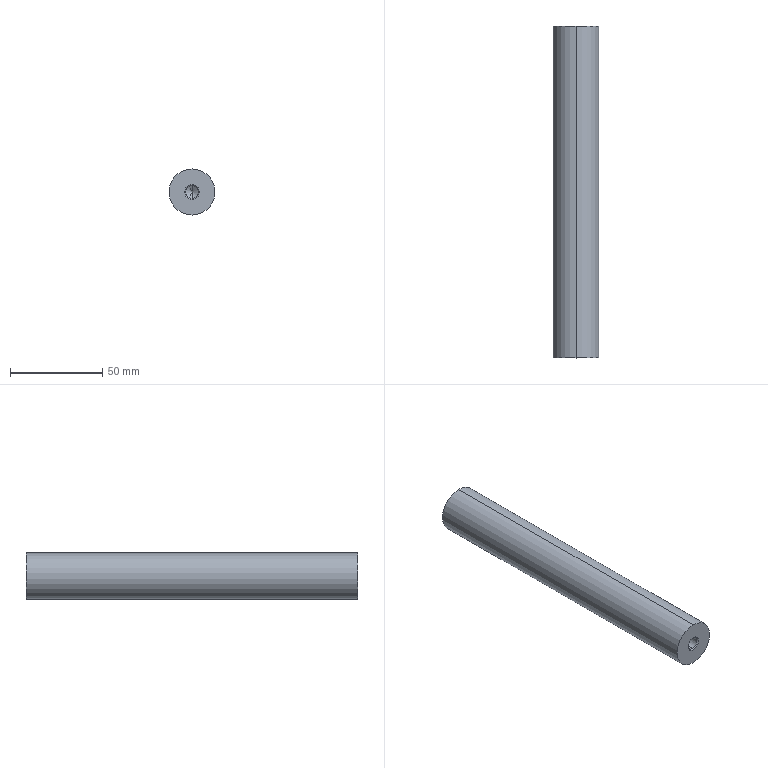Part | STEP file | A14-006 | 1 solid | 16 faces | box 25 x 180 x 25 mm | volume 86683 mm3 | cone 8 | cylinder 6 | plane 2 | commonest cylinder face diameters 6.8 x4 25 x2
STEP:
#1=CARTESIAN_POINT('',(0.,0.,0.));
#2=DIRECTION('',(0.,0.,1.));
#3=DIRECTION('',(1.,0.,0.));
#4=AXIS2_PLACEMENT_3D('',#1,#2,#3);
#5=CARTESIAN_POINT('',(0.,89.375,3.4));
#6=VERTEX_POINT('',#5);
#7=CARTESIAN_POINT('',(0.,90.,4.025));
#8=VERTEX_POINT('',#7);
#9=CARTESIAN_POINT('',(0.,90.,4.025));
#10=DIRECTION('',(0.,0.7071,0.7071));
#11=VECTOR('',#10,1.);
#12=LINE('',#9,#11);
#13=CARTESIAN_POINT('',(0.,90.,0.));
#14=DIRECTION('',(0.,1.,0.));
#15=DIRECTION('',(0.,0.,1.));
#16=AXIS2_PLACEMENT_3D('',#13,#14,#15);
#17=CONICAL_SURFACE('',#16,4.025,0.7854);
#18=CARTESIAN_POINT('',(6.283,0.));
#19=DIRECTION('',(0.,1.));
#20=VECTOR('',#19,1.);
#21=LINE('',#18,#20);
#22=(GEOMETRIC_REPRESENTATION_CONTEXT(2)PARAMETRIC_REPRESENTATION_CONTEXT()REPRESENTATION_CONTEXT('',''));
#23=DEFINITIONAL_REPRESENTATION('',(#21),#22);
#24=PCURVE('',#17,#23);
#25=CARTESIAN_POINT('',(0.,90.,0.));
#26=DIRECTION('',(0.,1.,0.));
#27=DIRECTION('',(0.,0.,1.));
#28=AXIS2_PLACEMENT_3D('',#25,#26,#27);
#29=CONICAL_SURFACE('',#28,4.025,0.7854);
#30=CARTESIAN_POINT('',(0.,0.));
#31=DIRECTION('',(0.,1.));
#32=VECTOR('',#31,1.);
#33=LINE('',#30,#32);
#34=(GEOMETRIC_REPRESENTATION_CONTEXT(2)PARAMETRIC_REPRESENTATION_CONTEXT()REPRESENTATION_CONTEXT('',''));
#35=DEFINITIONAL_REPRESENTATION('',(#33),#34);
#36=PCURVE('',#29,#35);
#37=SURFACE_CURVE('',#12,(#24,#36),.PCURVE_S1.);
#38=EDGE_CURVE('',#6,#8,#37,.T.);
#39=ORIENTED_EDGE('',*,*,#38,.T.);
#40=CARTESIAN_POINT('',(0.,90.,-4.025));
#41=VERTEX_POINT('',#40);
#42=CARTESIAN_POINT('',(0.,90.,0.));
#43=DIRECTION('',(0.,1.,0.));
#44=DIRECTION('',(0.,0.,1.));
#45=AXIS2_PLACEMENT_3D('',#42,#43,#44);
#46=CIRCLE('',#45,4.025);
#47=CARTESIAN_POINT('',(0.,0.));
#48=DIRECTION('',(1.,0.));
#49=VECTOR('',#48,1.);
#50=LINE('',#47,#49);
#51=(GEOMETRIC_REPRESENTATION_CONTEXT(2)PARAMETRIC_REPRESENTATION_CONTEXT()REPRESENTATION_CONTEXT('',''));
#52=DEFINITIONAL_REPRESENTATION('',(#50),#51);
#53=PCURVE('',#17,#52);
#54=CARTESIAN_POINT('',(0.,90.,0.));
#55=DIRECTION('',(0.,1.,0.));
#56=DIRECTION('',(0.,0.,1.));
#57=AXIS2_PLACEMENT_3D('',#54,#55,#56);
#58=PLANE('',#57);
#59=CARTESIAN_POINT('',(0.,0.));
#60=DIRECTION('',(1.,0.));
#61=AXIS2_PLACEMENT_2D('',#59,#60);
#62=CIRCLE('',#61,4.025);
#63=(GEOMETRIC_REPRESENTATION_CONTEXT(2)PARAMETRIC_REPRESENTATION_CONTEXT()REPRESENTATION_CONTEXT('',''));
#64=DEFINITIONAL_REPRESENTATION('',(#62),#63);
#65=PCURVE('',#58,#64);
#66=SURFACE_CURVE('',#46,(#53,#65),.PCURVE_S1.);
#67=EDGE_CURVE('',#41,#8,#66,.T.);
#68=ORIENTED_EDGE('',*,*,#67,.F.);
#69=CARTESIAN_POINT('',(0.,89.375,-3.4));
#70=VERTEX_POINT('',#69);
#71=CARTESIAN_POINT('',(0.,90.,-4.025));
#72=DIRECTION('',(0.,0.7071,-0.7071));
#73=VECTOR('',#72,1.);
#74=LINE('',#71,#73);
#75=CARTESIAN_POINT('',(3.142,0.));
#76=DIRECTION('',(0.,1.));
#77=VECTOR('',#76,1.);
#78=LINE('',#75,#77);
#79=(GEOMETRIC_REPRESENTATION_CONTEXT(2)PARAMETRIC_REPRESENTATION_CONTEXT()REPRESENTATION_CONTEXT('',''));
#80=DEFINITIONAL_REPRESENTATION('',(#78),#79);
#81=PCURVE('',#17,#80);
#82=CARTESIAN_POINT('',(3.142,0.));
#83=DIRECTION('',(0.,1.));
#84=VECTOR('',#83,1.);
#85=LINE('',#82,#84);
#86=(GEOMETRIC_REPRESENTATION_CONTEXT(2)PARAMETRIC_REPRESENTATION_CONTEXT()REPRESENTATION_CONTEXT('',''));
#87=DEFINITIONAL_REPRESENTATION('',(#85),#86);
#88=PCURVE('',#29,#87);
#89=SURFACE_CURVE('',#74,(#81,#88),.PCURVE_S1.);
#90=EDGE_CURVE('',#70,#41,#89,.T.);
#91=ORIENTED_EDGE('',*,*,#90,.F.);
#92=CARTESIAN_POINT('',(0.,89.375,0.));
#93=DIRECTION('',(0.,1.,0.));
#94=DIRECTION('',(0.,0.,1.));
#95=AXIS2_PLACEMENT_3D('',#92,#93,#94);
#96=CIRCLE('',#95,3.4);
#97=CARTESIAN_POINT('',(0.,-0.625));
#98=DIRECTION('',(1.,0.));
#99=VECTOR('',#98,1.);
#100=LINE('',#97,#99);
#101=(GEOMETRIC_REPRESENTATION_CONTEXT(2)PARAMETRIC_REPRESENTATION_CONTEXT()REPRESENTATION_CONTEXT('',''));
#102=DEFINITIONAL_REPRESENTATION('',(#100),#101);
#103=PCURVE('',#17,#102);
#104=CARTESIAN_POINT('',(0.,90.,0.));
#105=DIRECTION('',(0.,1.,0.));
#106=DIRECTION('',(0.,0.,1.));
#107=AXIS2_PLACEMENT_3D('',#104,#105,#106);
#108=CYLINDRICAL_SURFACE('',#107,3.4);
#109=CARTESIAN_POINT('',(0.,-0.625));
#110=DIRECTION('',(1.,0.));
#111=VECTOR('',#110,1.);
#112=LINE('',#109,#111);
#113=(GEOMETRIC_REPRESENTATION_CONTEXT(2)PARAMETRIC_REPRESENTATION_CONTEXT()REPRESENTATION_CONTEXT('',''));
#114=DEFINITIONAL_REPRESENTATION('',(#112),#113);
#115=PCURVE('',#108,#114);
#116=SURFACE_CURVE('',#96,(#103,#115),.PCURVE_S1.);
#117=EDGE_CURVE('',#70,#6,#116,.T.);
#118=ORIENTED_EDGE('',*,*,#117,.T.);
#119=EDGE_LOOP('',(#39,#68,#91,#118));
#120=FACE_BOUND('',#119,.F.);
#121=ADVANCED_FACE('',(#120),#17,.F.);
#122=CARTESIAN_POINT('',(0.,67.75,3.4));
#123=VERTEX_POINT('',#122);
#124=CARTESIAN_POINT('',(0.,90.,3.4));
#125=DIRECTION('',(0.,1.,0.));
#126=VECTOR('',#125,1.);
#127=LINE('',#124,#126);
#128=CARTESIAN_POINT('',(6.283,0.));
#129=DIRECTION('',(0.,1.));
#130=VECTOR('',#129,1.);
#131=LINE('',#128,#130);
#132=(GEOMETRIC_REPRESENTATION_CONTEXT(2)PARAMETRIC_REPRESENTATION_CONTEXT()REPRESENTATION_CONTEXT('',''));
#133=DEFINITIONAL_REPRESENTATION('',(#131),#132);
#134=PCURVE('',#108,#133);
#135=CARTESIAN_POINT('',(0.,90.,0.));
#136=DIRECTION('',(0.,1.,0.));
#137=DIRECTION('',(0.,0.,1.));
#138=AXIS2_PLACEMENT_3D('',#135,#136,#137);
#139=CYLINDRICAL_SURFACE('',#138,3.4);
#140=CARTESIAN_POINT('',(0.,0.));
#141=DIRECTION('',(0.,1.));
#142=VECTOR('',#141,1.);
#143=LINE('',#140,#142);
#144=(GEOMETRIC_REPRESENTATION_CONTEXT(2)PARAMETRIC_REPRESENTATION_CONTEXT()REPRESENTATION_CONTEXT('',''));
#145=DEFINITIONAL_REPRESENTATION('',(#143),#144);
#146=PCURVE('',#139,#145);
#147=SURFACE_CURVE('',#127,(#134,#146),.PCURVE_S1.);
#148=EDGE_CURVE('',#123,#6,#147,.T.);
#149=ORIENTED_EDGE('',*,*,#148,.T.);
#150=ORIENTED_EDGE('',*,*,#117,.F.);
#151=CARTESIAN_POINT('',(0.,67.75,-3.4));
#152=VERTEX_POINT('',#151);
#153=CARTESIAN_POINT('',(0.,90.,-3.4));
#154=DIRECTION('',(0.,1.,0.));
#155=VECTOR('',#154,1.);
#156=LINE('',#153,#155);
#157=CARTESIAN_POINT('',(3.142,0.));
#158=DIRECTION('',(0.,1.));
#159=VECTOR('',#158,1.);
#160=LINE('',#157,#159);
#161=(GEOMETRIC_REPRESENTATION_CONTEXT(2)PARAMETRIC_REPRESENTATION_CONTEXT()REPRESENTATION_CONTEXT('',''));
#162=DEFINITIONAL_REPRESENTATION('',(#160),#161);
#163=PCURVE('',#108,#162);
#164=CARTESIAN_POINT('',(3.142,0.));
#165=DIRECTION('',(0.,1.));
#166=VECTOR('',#165,1.);
#167=LINE('',#164,#166);
#168=(GEOMETRIC_REPRESENTATION_CONTEXT(2)PARAMETRIC_REPRESENTATION_CONTEXT()REPRESENTATION_CONTEXT('',''));
#169=DEFINITIONAL_REPRESENTATION('',(#167),#168);
#170=PCURVE('',#139,#169);
#171=SURFACE_CURVE('',#156,(#163,#170),.PCURVE_S1.);
#172=EDGE_CURVE('',#152,#70,#171,.T.);
#173=ORIENTED_EDGE('',*,*,#172,.F.);
#174=CARTESIAN_POINT('',(0.,67.75,0.));
#175=DIRECTION('',(0.,1.,0.));
#176=DIRECTION('',(0.,0.,1.));
#177=AXIS2_PLACEMENT_3D('',#174,#175,#176);
#178=CIRCLE('',#177,3.4);
#179=CARTESIAN_POINT('',(0.,-22.25));
#180=DIRECTION('',(1.,0.));
#181=VECTOR('',#180,1.);
#182=LINE('',#179,#181);
#183=(GEOMETRIC_REPRESENTATION_CONTEXT(2)PARAMETRIC_REPRESENTATION_CONTEXT()REPRESENTATION_CONTEXT('',''));
#184=DEFINITIONAL_REPRESENTATION('',(#182),#183);
#185=PCURVE('',#108,#184);
#186=CARTESIAN_POINT('',(0.,67.75,0.));
#187=DIRECTION('',(0.,1.,0.));
#188=DIRECTION('',(0.,0.,1.));
#189=AXIS2_PLACEMENT_3D('',#186,#187,#188);
#190=CONICAL_SURFACE('',#189,3.4,1.03);
#191=CARTESIAN_POINT('',(0.,0.));
#192=DIRECTION('',(1.,0.));
#193=VECTOR('',#192,1.);
#194=LINE('',#191,#193);
#195=(GEOMETRIC_REPRESENTATION_CONTEXT(2)PARAMETRIC_REPRESENTATION_CONTEXT()REPRESENTATION_CONTEXT('',''));
#196=DEFINITIONAL_REPRESENTATION('',(#194),#195);
#197=PCURVE('',#190,#196);
#198=SURFACE_CURVE('',#178,(#185,#197),.PCURVE_S1.);
#199=EDGE_CURVE('',#152,#123,#198,.T.);
#200=ORIENTED_EDGE('',*,*,#199,.T.);
#201=EDGE_LOOP('',(#149,#150,#173,#200));
#202=FACE_BOUND('',#201,.F.);
#203=ADVANCED_FACE('',(#202),#108,.F.);
#204=ORIENTED_EDGE('',*,*,#199,.F.);
#205=CARTESIAN_POINT('',(0.,65.707,0.));
#206=VERTEX_POINT('',#205);
#207=CARTESIAN_POINT('',(0.,67.75,-3.4));
#208=DIRECTION('',(0.,0.515,-0.8572));
#209=VECTOR('',#208,1.);
#210=LINE('',#207,#209);
#211=CARTESIAN_POINT('',(3.142,-2.043));
#212=CARTESIAN_POINT('',(3.142,-2.012));
#213=CARTESIAN_POINT('',(3.142,-1.95));
#214=CARTESIAN_POINT('',(3.142,-1.857));
#215=CARTESIAN_POINT('',(3.142,-1.764));
#216=CARTESIAN_POINT('',(3.142,-1.671));
#217=CARTESIAN_POINT('',(3.142,-1.579));
#218=CARTESIAN_POINT('',(3.142,-1.486));
#219=CARTESIAN_POINT('',(3.142,-1.393));
#220=CARTESIAN_POINT('',(3.142,-1.3));
#221=CARTESIAN_POINT('',(3.142,-1.207));
#222=CARTESIAN_POINT('',(3.142,-1.114));
#223=CARTESIAN_POINT('',(3.142,-1.021));
#224=CARTESIAN_POINT('',(3.142,-0.9286));
#225=CARTESIAN_POINT('',(3.142,-0.8357));
#226=CARTESIAN_POINT('',(3.142,-0.7429));
#227=CARTESIAN_POINT('',(3.142,-0.65));
#228=CARTESIAN_POINT('',(3.142,-0.5572));
#229=CARTESIAN_POINT('',(3.142,-0.4643));
#230=CARTESIAN_POINT('',(3.142,-0.3714));
#231=CARTESIAN_POINT('',(3.142,-0.2786));
#232=CARTESIAN_POINT('',(3.142,-0.1857));
#233=CARTESIAN_POINT('',(3.142,-0.09286));
#234=CARTESIAN_POINT('',(3.142,-0.03095));
#235=CARTESIAN_POINT('',(3.142,0.));
#236=B_SPLINE_CURVE_WITH_KNOTS('',3,(#211,#212,#213,#214,#215,#216,#217,#218,#219,#220,#221,#222,#223,#224,#225,#226,#227,#228,#229,#230,#231,#232,#233,#234,#235),.UNSPECIFIED.,.F.,.F.,(4,1,1,1,1,1,1,1,1,1,1,1,1,1,1,1,1,1,1,1,1,1,4),(-3.967,-3.786,-3.606,-3.426,-3.245,-3.065,-2.885,-2.704,-2.524,-2.344,-2.164,-1.983,-1.803,-1.623,-1.442,-1.262,-1.082,-0.9015,-0.7212,-0.5409,-0.3606,-0.1803,0.),.UNSPECIFIED.);
#237=(GEOMETRIC_REPRESENTATION_CONTEXT(2)PARAMETRIC_REPRESENTATION_CONTEXT()REPRESENTATION_CONTEXT('',''));
#238=DEFINITIONAL_REPRESENTATION('',(#236),#237);
#239=PCURVE('',#190,#238);
#240=CARTESIAN_POINT('',(0.,67.75,0.));
#241=DIRECTION('',(0.,1.,0.));
#242=DIRECTION('',(0.,0.,1.));
#243=AXIS2_PLACEMENT_3D('',#240,#241,#242);
#244=CONICAL_SURFACE('',#243,3.4,1.03);
#245=CARTESIAN_POINT('',(3.142,-2.043));
#246=CARTESIAN_POINT('',(3.142,-2.012));
#247=CARTESIAN_POINT('',(3.142,-1.95));
#248=CARTESIAN_POINT('',(3.142,-1.857));
#249=CARTESIAN_POINT('',(3.142,-1.764));
#250=CARTESIAN_POINT('',(3.142,-1.671));
#251=CARTESIAN_POINT('',(3.142,-1.579));
#252=CARTESIAN_POINT('',(3.142,-1.486));
#253=CARTESIAN_POINT('',(3.142,-1.393));
#254=CARTESIAN_POINT('',(3.142,-1.3));
#255=CARTESIAN_POINT('',(3.142,-1.207));
#256=CARTESIAN_POINT('',(3.142,-1.114));
#257=CARTESIAN_POINT('',(3.142,-1.021));
#258=CARTESIAN_POINT('',(3.142,-0.9286));
#259=CARTESIAN_POINT('',(3.142,-0.8357));
#260=CARTESIAN_POINT('',(3.142,-0.7429));
#261=CARTESIAN_POINT('',(3.142,-0.65));
#262=CARTESIAN_POINT('',(3.142,-0.5572));
#263=CARTESIAN_POINT('',(3.142,-0.4643));
#264=CARTESIAN_POINT('',(3.142,-0.3714));
#265=CARTESIAN_POINT('',(3.142,-0.2786));
#266=CARTESIAN_POINT('',(3.142,-0.1857));
#267=CARTESIAN_POINT('',(3.142,-0.09286));
#268=CARTESIAN_POINT('',(3.142,-0.03095));
#269=CARTESIAN_POINT('',(3.142,0.));
#270=B_SPLINE_CURVE_WITH_KNOTS('',3,(#245,#246,#247,#248,#249,#250,#251,#252,#253,#254,#255,#256,#257,#258,#259,#260,#261,#262,#263,#264,#265,#266,#267,#268,#269),.UNSPECIFIED.,.F.,.F.,(4,1,1,1,1,1,1,1,1,1,1,1,1,1,1,1,1,1,1,1,1,1,4),(-3.967,-3.786,-3.606,-3.426,-3.245,-3.065,-2.885,-2.704,-2.524,-2.344,-2.164,-1.983,-1.803,-1.623,-1.442,-1.262,-1.082,-0.9015,-0.7212,-0.5409,-0.3606,-0.1803,0.),.UNSPECIFIED.);
#271=(GEOMETRIC_REPRESENTATION_CONTEXT(2)PARAMETRIC_REPRESENTATION_CONTEXT()REPRESENTATION_CONTEXT('',''));
#272=DEFINITIONAL_REPRESENTATION('',(#270),#271);
#273=PCURVE('',#244,#272);
#274=SURFACE_CURVE('',#210,(#239,#273),.PCURVE_S1.);
#275=EDGE_CURVE('',#206,#152,#274,.T.);
#276=ORIENTED_EDGE('',*,*,#275,.F.);
#277=CARTESIAN_POINT('',(0.,67.75,3.4));
#278=DIRECTION('',(0.,0.515,0.8572));
#279=VECTOR('',#278,1.);
#280=LINE('',#277,#279);
#281=CARTESIAN_POINT('',(6.283,-2.043));
#282=CARTESIAN_POINT('',(6.283,-2.012));
#283=CARTESIAN_POINT('',(6.283,-1.95));
#284=CARTESIAN_POINT('',(6.283,-1.857));
#285=CARTESIAN_POINT('',(6.283,-1.764));
#286=CARTESIAN_POINT('',(6.283,-1.671));
#287=CARTESIAN_POINT('',(6.283,-1.579));
#288=CARTESIAN_POINT('',(6.283,-1.486));
#289=CARTESIAN_POINT('',(6.283,-1.393));
#290=CARTESIAN_POINT('',(6.283,-1.3));
#291=CARTESIAN_POINT('',(6.283,-1.207));
#292=CARTESIAN_POINT('',(6.283,-1.114));
#293=CARTESIAN_POINT('',(6.283,-1.021));
#294=CARTESIAN_POINT('',(6.283,-0.9286));
#295=CARTESIAN_POINT('',(6.283,-0.8357));
#296=CARTESIAN_POINT('',(6.283,-0.7429));
#297=CARTESIAN_POINT('',(6.283,-0.65));
#298=CARTESIAN_POINT('',(6.283,-0.5572));
#299=CARTESIAN_POINT('',(6.283,-0.4643));
#300=CARTESIAN_POINT('',(6.283,-0.3714));
#301=CARTESIAN_POINT('',(6.283,-0.2786));
#302=CARTESIAN_POINT('',(6.283,-0.1857));
#303=CARTESIAN_POINT('',(6.283,-0.09286));
#304=CARTESIAN_POINT('',(6.283,-0.03095));
#305=CARTESIAN_POINT('',(6.283,0.));
#306=B_SPLINE_CURVE_WITH_KNOTS('',3,(#281,#282,#283,#284,#285,#286,#287,#288,#289,#290,#291,#292,#293,#294,#295,#296,#297,#298,#299,#300,#301,#302,#303,#304,#305),.UNSPECIFIED.,.F.,.F.,(4,1,1,1,1,1,1,1,1,1,1,1,1,1,1,1,1,1,1,1,1,1,4),(-3.967,-3.786,-3.606,-3.426,-3.245,-3.065,-2.885,-2.704,-2.524,-2.344,-2.164,-1.983,-1.803,-1.623,-1.442,-1.262,-1.082,-0.9015,-0.7212,-0.5409,-0.3606,-0.1803,0.),.UNSPECIFIED.);
#307=(GEOMETRIC_REPRESENTATION_CONTEXT(2)PARAMETRIC_REPRESENTATION_CONTEXT()REPRESENTATION_CONTEXT('',''));
#308=DEFINITIONAL_REPRESENTATION('',(#306),#307);
#309=PCURVE('',#190,#308);
#310=CARTESIAN_POINT('',(0.,-2.043));
#311=CARTESIAN_POINT('',(0.,-2.012));
#312=CARTESIAN_POINT('',(0.,-1.95));
#313=CARTESIAN_POINT('',(0.,-1.857));
#314=CARTESIAN_POINT('',(0.,-1.764));
#315=CARTESIAN_POINT('',(0.,-1.671));
#316=CARTESIAN_POINT('',(0.,-1.579));
#317=CARTESIAN_POINT('',(0.,-1.486));
#318=CARTESIAN_POINT('',(0.,-1.393));
#319=CARTESIAN_POINT('',(0.,-1.3));
#320=CARTESIAN_POINT('',(0.,-1.207));
#321=CARTESIAN_POINT('',(0.,-1.114));
#322=CARTESIAN_POINT('',(0.,-1.021));
#323=CARTESIAN_POINT('',(0.,-0.9286));
#324=CARTESIAN_POINT('',(0.,-0.8357));
#325=CARTESIAN_POINT('',(0.,-0.7429));
#326=CARTESIAN_POINT('',(0.,-0.65));
#327=CARTESIAN_POINT('',(0.,-0.5572));
#328=CARTESIAN_POINT('',(0.,-0.4643));
#329=CARTESIAN_POINT('',(0.,-0.3714));
#330=CARTESIAN_POINT('',(0.,-0.2786));
#331=CARTESIAN_POINT('',(0.,-0.1857));
#332=CARTESIAN_POINT('',(0.,-0.09286));
#333=CARTESIAN_POINT('',(0.,-0.03095));
#334=CARTESIAN_POINT('',(0.,0.));
#335=B_SPLINE_CURVE_WITH_KNOTS('',3,(#310,#311,#312,#313,#314,#315,#316,#317,#318,#319,#320,#321,#322,#323,#324,#325,#326,#327,#328,#329,#330,#331,#332,#333,#334),.UNSPECIFIED.,.F.,.F.,(4,1,1,1,1,1,1,1,1,1,1,1,1,1,1,1,1,1,1,1,1,1,4),(-3.967,-3.786,-3.606,-3.426,-3.245,-3.065,-2.885,-2.704,-2.524,-2.344,-2.164,-1.983,-1.803,-1.623,-1.442,-1.262,-1.082,-0.9015,-0.7212,-0.5409,-0.3606,-0.1803,0.),.UNSPECIFIED.);
#336=(GEOMETRIC_REPRESENTATION_CONTEXT(2)PARAMETRIC_REPRESENTATION_CONTEXT()REPRESENTATION_CONTEXT('',''));
#337=DEFINITIONAL_REPRESENTATION('',(#335),#336);
#338=PCURVE('',#244,#337);
#339=SURFACE_CURVE('',#280,(#309,#338),.PCURVE_S1.);
#340=EDGE_CURVE('',#206,#123,#339,.T.);
#341=ORIENTED_EDGE('',*,*,#340,.T.);
#342=EDGE_LOOP('',(#204,#276,#341));
#343=FACE_BOUND('',#342,.F.);
#344=ADVANCED_FACE('',(#343),#190,.F.);
#345=CARTESIAN_POINT('',(0.,-89.375,-3.4));
#346=VERTEX_POINT('',#345);
#347=CARTESIAN_POINT('',(0.,-90.,-4.025));
#348=VERTEX_POINT('',#347);
#349=CARTESIAN_POINT('',(0.,-90.,-4.025));
#350=DIRECTION('',(0.,-0.7071,-0.7071));
#351=VECTOR('',#350,1.);
#352=LINE('',#349,#351);
#353=CARTESIAN_POINT('',(0.,-90.,0.));
#354=DIRECTION('',(0.,-1.,0.));
#355=DIRECTION('',(0.,0.,-1.));
#356=AXIS2_PLACEMENT_3D('',#353,#354,#355);
#357=CONICAL_SURFACE('',#356,4.025,0.7854);
#358=CARTESIAN_POINT('',(6.283,0.));
#359=DIRECTION('',(0.,1.));
#360=VECTOR('',#359,1.);
#361=LINE('',#358,#360);
#362=(GEOMETRIC_REPRESENTATION_CONTEXT(2)PARAMETRIC_REPRESENTATION_CONTEXT()REPRESENTATION_CONTEXT('',''));
#363=DEFINITIONAL_REPRESENTATION('',(#361),#362);
#364=PCURVE('',#357,#363);
#365=CARTESIAN_POINT('',(0.,-90.,0.));
#366=DIRECTION('',(0.,-1.,0.));
#367=DIRECTION('',(0.,0.,-1.));
#368=AXIS2_PLACEMENT_3D('',#365,#366,#367);
#369=CONICAL_SURFACE('',#368,4.025,0.7854);
#370=CARTESIAN_POINT('',(0.,0.));
#371=DIRECTION('',(0.,1.));
#372=VECTOR('',#371,1.);
#373=LINE('',#370,#372);
#374=(GEOMETRIC_REPRESENTATION_CONTEXT(2)PARAMETRIC_REPRESENTATION_CONTEXT()REPRESENTATION_CONTEXT('',''));
#375=DEFINITIONAL_REPRESENTATION('',(#373),#374);
#376=PCURVE('',#369,#375);
#377=SURFACE_CURVE('',#352,(#364,#376),.PCURVE_S1.);
#378=EDGE_CURVE('',#346,#348,#377,.T.);
#379=ORIENTED_EDGE('',*,*,#378,.T.);
#380=CARTESIAN_POINT('',(0.,-90.,4.025));
#381=VERTEX_POINT('',#380);
#382=CARTESIAN_POINT('',(0.,-90.,0.));
#383=DIRECTION('',(0.,-1.,0.));
#384=DIRECTION('',(0.,0.,-1.));
#385=AXIS2_PLACEMENT_3D('',#382,#383,#384);
#386=CIRCLE('',#385,4.025);
#387=CARTESIAN_POINT('',(0.,0.));
#388=DIRECTION('',(1.,0.));
#389=VECTOR('',#388,1.);
#390=LINE('',#387,#389);
#391=(GEOMETRIC_REPRESENTATION_CONTEXT(2)PARAMETRIC_REPRESENTATION_CONTEXT()REPRESENTATION_CONTEXT('',''));
#392=DEFINITIONAL_REPRESENTATION('',(#390),#391);
#393=PCURVE('',#357,#392);
#394=CARTESIAN_POINT('',(0.,-90.,0.));
#395=DIRECTION('',(0.,1.,0.));
#396=DIRECTION('',(0.,0.,1.));
#397=AXIS2_PLACEMENT_3D('',#394,#395,#396);
#398=PLANE('',#397);
#399=CARTESIAN_POINT('',(-4.025,0.));
#400=CARTESIAN_POINT('',(-4.025,6.972));
#401=CARTESIAN_POINT('',(2.013,3.486));
#402=CARTESIAN_POINT('',(8.05,0.));
#403=CARTESIAN_POINT('',(2.013,-3.486));
#404=CARTESIAN_POINT('',(-4.025,-6.972));
#405=CARTESIAN_POINT('',(-4.025,0.));
#406=(BOUNDED_CURVE()B_SPLINE_CURVE(2,(#399,#400,#401,#402,#403,#404,#405),.UNSPECIFIED.,.T.,.F.)B_SPLINE_CURVE_WITH_KNOTS((1,2,2,2,2,1),(-2.094,0.,2.094,4.189,6.283,8.378),.UNSPECIFIED.)CURVE()GEOMETRIC_REPRESENTATION_ITEM()RATIONAL_B_SPLINE_CURVE((1.,0.5,1.,0.5,1.,0.5,1.))REPRESENTATION_ITEM(''));
#407=(GEOMETRIC_REPRESENTATION_CONTEXT(2)PARAMETRIC_REPRESENTATION_CONTEXT()REPRESENTATION_CONTEXT('',''));
#408=DEFINITIONAL_REPRESENTATION('',(#406),#407);
#409=PCURVE('',#398,#408);
#410=SURFACE_CURVE('',#386,(#393,#409),.PCURVE_S1.);
#411=EDGE_CURVE('',#381,#348,#410,.T.);
#412=ORIENTED_EDGE('',*,*,#411,.F.);
#413=CARTESIAN_POINT('',(0.,-89.375,3.4));
#414=VERTEX_POINT('',#413);
#415=CARTESIAN_POINT('',(0.,-90.,4.025));
#416=DIRECTION('',(0.,-0.7071,0.7071));
#417=VECTOR('',#416,1.);
#418=LINE('',#415,#417);
#419=CARTESIAN_POINT('',(3.142,0.));
#420=DIRECTION('',(0.,1.));
#421=VECTOR('',#420,1.);
#422=LINE('',#419,#421);
#423=(GEOMETRIC_REPRESENTATION_CONTEXT(2)PARAMETRIC_REPRESENTATION_CONTEXT()REPRESENTATION_CONTEXT('',''));
#424=DEFINITIONAL_REPRESENTATION('',(#422),#423);
#425=PCURVE('',#357,#424);
#426=CARTESIAN_POINT('',(3.142,0.));
#427=DIRECTION('',(0.,1.));
#428=VECTOR('',#427,1.);
#429=LINE('',#426,#428);
#430=(GEOMETRIC_REPRESENTATION_CONTEXT(2)PARAMETRIC_REPRESENTATION_CONTEXT()REPRESENTATION_CONTEXT('',''));
#431=DEFINITIONAL_REPRESENTATION('',(#429),#430);
#432=PCURVE('',#369,#431);
#433=SURFACE_CURVE('',#418,(#425,#432),.PCURVE_S1.);
#434=EDGE_CURVE('',#414,#381,#433,.T.);
#435=ORIENTED_EDGE('',*,*,#434,.F.);
#436=CARTESIAN_POINT('',(0.,-89.375,0.));
#437=DIRECTION('',(0.,-1.,0.));
#438=DIRECTION('',(0.,0.,-1.));
#439=AXIS2_PLACEMENT_3D('',#436,#437,#438);
#440=CIRCLE('',#439,3.4);
#441=CARTESIAN_POINT('',(0.,-0.625));
#442=DIRECTION('',(1.,0.));
#443=VECTOR('',#442,1.);
#444=LINE('',#441,#443);
#445=(GEOMETRIC_REPRESENTATION_CONTEXT(2)PARAMETRIC_REPRESENTATION_CONTEXT()REPRESENTATION_CONTEXT('',''));
#446=DEFINITIONAL_REPRESENTATION('',(#444),#445);
#447=PCURVE('',#357,#446);
#448=CARTESIAN_POINT('',(0.,-90.,0.));
#449=DIRECTION('',(0.,-1.,0.));
#450=DIRECTION('',(0.,0.,-1.));
#451=AXIS2_PLACEMENT_3D('',#448,#449,#450);
#452=CYLINDRICAL_SURFACE('',#451,3.4);
#453=CARTESIAN_POINT('',(0.,-0.625));
#454=DIRECTION('',(1.,0.));
#455=VECTOR('',#454,1.);
#456=LINE('',#453,#455);
#457=(GEOMETRIC_REPRESENTATION_CONTEXT(2)PARAMETRIC_REPRESENTATION_CONTEXT()REPRESENTATION_CONTEXT('',''));
#458=DEFINITIONAL_REPRESENTATION('',(#456),#457);
#459=PCURVE('',#452,#458);
#460=SURFACE_CURVE('',#440,(#447,#459),.PCURVE_S1.);
#461=EDGE_CURVE('',#414,#346,#460,.T.);
#462=ORIENTED_EDGE('',*,*,#461,.T.);
#463=EDGE_LOOP('',(#379,#412,#435,#462));
#464=FACE_BOUND('',#463,.F.);
#465=ADVANCED_FACE('',(#464),#357,.F.);
#466=CARTESIAN_POINT('',(0.,-67.75,-3.4));
#467=VERTEX_POINT('',#466);
#468=CARTESIAN_POINT('',(0.,-90.,-3.4));
#469=DIRECTION('',(0.,-1.,0.));
#470=VECTOR('',#469,1.);
#471=LINE('',#468,#470);
#472=CARTESIAN_POINT('',(6.283,0.));
#473=DIRECTION('',(0.,1.));
#474=VECTOR('',#473,1.);
#475=LINE('',#472,#474);
#476=(GEOMETRIC_REPRESENTATION_CONTEXT(2)PARAMETRIC_REPRESENTATION_CONTEXT()REPRESENTATION_CONTEXT('',''));
#477=DEFINITIONAL_REPRESENTATION('',(#475),#476);
#478=PCURVE('',#452,#477);
#479=CARTESIAN_POINT('',(0.,-90.,0.));
#480=DIRECTION('',(0.,-1.,0.));
#481=DIRECTION('',(0.,0.,-1.));
#482=AXIS2_PLACEMENT_3D('',#479,#480,#481);
#483=CYLINDRICAL_SURFACE('',#482,3.4);
#484=CARTESIAN_POINT('',(0.,0.));
#485=DIRECTION('',(0.,1.));
#486=VECTOR('',#485,1.);
#487=LINE('',#484,#486);
#488=(GEOMETRIC_REPRESENTATION_CONTEXT(2)PARAMETRIC_REPRESENTATION_CONTEXT()REPRESENTATION_CONTEXT('',''));
#489=DEFINITIONAL_REPRESENTATION('',(#487),#488);
#490=PCURVE('',#483,#489);
#491=SURFACE_CURVE('',#471,(#478,#490),.PCURVE_S1.);
#492=EDGE_CURVE('',#467,#346,#491,.T.);
#493=ORIENTED_EDGE('',*,*,#492,.T.);
#494=ORIENTED_EDGE('',*,*,#461,.F.);
#495=CARTESIAN_POINT('',(0.,-67.75,3.4));
#496=VERTEX_POINT('',#495);
#497=CARTESIAN_POINT('',(0.,-90.,3.4));
#498=DIRECTION('',(0.,-1.,0.));
#499=VECTOR('',#498,1.);
#500=LINE('',#497,#499);
#501=CARTESIAN_POINT('',(3.142,0.));
#502=DIRECTION('',(0.,1.));
#503=VECTOR('',#502,1.);
#504=LINE('',#501,#503);
#505=(GEOMETRIC_REPRESENTATION_CONTEXT(2)PARAMETRIC_REPRESENTATION_CONTEXT()REPRESENTATION_CONTEXT('',''));
#506=DEFINITIONAL_REPRESENTATION('',(#504),#505);
#507=PCURVE('',#452,#506);
#508=CARTESIAN_POINT('',(3.142,0.));
#509=DIRECTION('',(0.,1.));
#510=VECTOR('',#509,1.);
#511=LINE('',#508,#510);
#512=(GEOMETRIC_REPRESENTATION_CONTEXT(2)PARAMETRIC_REPRESENTATION_CONTEXT()REPRESENTATION_CONTEXT('',''));
#513=DEFINITIONAL_REPRESENTATION('',(#511),#512);
#514=PCURVE('',#483,#513);
#515=SURFACE_CURVE('',#500,(#507,#514),.PCURVE_S1.);
#516=EDGE_CURVE('',#496,#414,#515,.T.);
#517=ORIENTED_EDGE('',*,*,#516,.F.);
#518=CARTESIAN_POINT('',(0.,-67.75,0.));
#519=DIRECTION('',(0.,-1.,0.));
#520=DIRECTION('',(0.,0.,-1.));
#521=AXIS2_PLACEMENT_3D('',#518,#519,#520);
#522=CIRCLE('',#521,3.4);
#523=CARTESIAN_POINT('',(0.,-22.25));
#524=DIRECTION('',(1.,0.));
#525=VECTOR('',#524,1.);
#526=LINE('',#523,#525);
#527=(GEOMETRIC_REPRESENTATION_CONTEXT(2)PARAMETRIC_REPRESENTATION_CONTEXT()REPRESENTATION_CONTEXT('',''));
#528=DEFINITIONAL_REPRESENTATION('',(#526),#527);
#529=PCURVE('',#452,#528);
#530=CARTESIAN_POINT('',(0.,-67.75,0.));
#531=DIRECTION('',(0.,-1.,0.));
#532=DIRECTION('',(0.,0.,-1.));
#533=AXIS2_PLACEMENT_3D('',#530,#531,#532);
#534=CONICAL_SURFACE('',#533,3.4,1.03);
#535=CARTESIAN_POINT('',(0.,0.));
#536=DIRECTION('',(1.,0.));
#537=VECTOR('',#536,1.);
#538=LINE('',#535,#537);
#539=(GEOMETRIC_REPRESENTATION_CONTEXT(2)PARAMETRIC_REPRESENTATION_CONTEXT()REPRESENTATION_CONTEXT('',''));
#540=DEFINITIONAL_REPRESENTATION('',(#538),#539);
#541=PCURVE('',#534,#540);
#542=SURFACE_CURVE('',#522,(#529,#541),.PCURVE_S1.);
#543=EDGE_CURVE('',#496,#467,#542,.T.);
#544=ORIENTED_EDGE('',*,*,#543,.T.);
#545=EDGE_LOOP('',(#493,#494,#517,#544));
#546=FACE_BOUND('',#545,.F.);
#547=ADVANCED_FACE('',(#546),#452,.F.);
#548=ORIENTED_EDGE('',*,*,#543,.F.);
#549=CARTESIAN_POINT('',(0.,-65.707,0.));
#550=VERTEX_POINT('',#549);
#551=CARTESIAN_POINT('',(0.,-67.75,3.4));
#552=DIRECTION('',(0.,-0.515,0.8572));
#553=VECTOR('',#552,1.);
#554=LINE('',#551,#553);
#555=CARTESIAN_POINT('',(3.142,-2.043));
#556=CARTESIAN_POINT('',(3.142,-2.012));
#557=CARTESIAN_POINT('',(3.142,-1.95));
#558=CARTESIAN_POINT('',(3.142,-1.857));
#559=CARTESIAN_POINT('',(3.142,-1.764));
#560=CARTESIAN_POINT('',(3.142,-1.671));
#561=CARTESIAN_POINT('',(3.142,-1.579));
#562=CARTESIAN_POINT('',(3.142,-1.486));
#563=CARTESIAN_POINT('',(3.142,-1.393));
#564=CARTESIAN_POINT('',(3.142,-1.3));
#565=CARTESIAN_POINT('',(3.142,-1.207));
#566=CARTESIAN_POINT('',(3.142,-1.114));
#567=CARTESIAN_POINT('',(3.142,-1.021));
#568=CARTESIAN_POINT('',(3.142,-0.9286));
#569=CARTESIAN_POINT('',(3.142,-0.8357));
#570=CARTESIAN_POINT('',(3.142,-0.7429));
#571=CARTESIAN_POINT('',(3.142,-0.65));
#572=CARTESIAN_POINT('',(3.142,-0.5572));
#573=CARTESIAN_POINT('',(3.142,-0.4643));
#574=CARTESIAN_POINT('',(3.142,-0.3714));
#575=CARTESIAN_POINT('',(3.142,-0.2786));
#576=CARTESIAN_POINT('',(3.142,-0.1857));
#577=CARTESIAN_POINT('',(3.142,-0.09286));
#578=CARTESIAN_POINT('',(3.142,-0.03095));
#579=CARTESIAN_POINT('',(3.142,0.));
#580=B_SPLINE_CURVE_WITH_KNOTS('',3,(#555,#556,#557,#558,#559,#560,#561,#562,#563,#564,#565,#566,#567,#568,#569,#570,#571,#572,#573,#574,#575,#576,#577,#578,#579),.UNSPECIFIED.,.F.,.F.,(4,1,1,1,1,1,1,1,1,1,1,1,1,1,1,1,1,1,1,1,1,1,4),(-3.967,-3.786,-3.606,-3.426,-3.245,-3.065,-2.885,-2.704,-2.524,-2.344,-2.164,-1.983,-1.803,-1.623,-1.442,-1.262,-1.082,-0.9015,-0.7212,-0.5409,-0.3606,-0.1803,0.),.UNSPECIFIED.);
#581=(GEOMETRIC_REPRESENTATION_CONTEXT(2)PARAMETRIC_REPRESENTATION_CONTEXT()REPRESENTATION_CONTEXT('',''));
#582=DEFINITIONAL_REPRESENTATION('',(#580),#581);
#583=PCURVE('',#534,#582);
#584=CARTESIAN_POINT('',(0.,-67.75,0.));
#585=DIRECTION('',(0.,-1.,0.));
#586=DIRECTION('',(0.,0.,-1.));
#587=AXIS2_PLACEMENT_3D('',#584,#585,#586);
#588=CONICAL_SURFACE('',#587,3.4,1.03);
#589=CARTESIAN_POINT('',(3.142,-2.043));
#590=CARTESIAN_POINT('',(3.142,-2.012));
#591=CARTESIAN_POINT('',(3.142,-1.95));
#592=CARTESIAN_POINT('',(3.142,-1.857));
#593=CARTESIAN_POINT('',(3.142,-1.764));
#594=CARTESIAN_POINT('',(3.142,-1.671));
#595=CARTESIAN_POINT('',(3.142,-1.579));
#596=CARTESIAN_POINT('',(3.142,-1.486));
#597=CARTESIAN_POINT('',(3.142,-1.393));
#598=CARTESIAN_POINT('',(3.142,-1.3));
#599=CARTESIAN_POINT('',(3.142,-1.207));
#600=CARTESIAN_POINT('',(3.142,-1.114));
#601=CARTESIAN_POINT('',(3.142,-1.021));
#602=CARTESIAN_POINT('',(3.142,-0.9286));
#603=CARTESIAN_POINT('',(3.142,-0.8357));
#604=CARTESIAN_POINT('',(3.142,-0.7429));
#605=CARTESIAN_POINT('',(3.142,-0.65));
#606=CARTESIAN_POINT('',(3.142,-0.5572));
#607=CARTESIAN_POINT('',(3.142,-0.4643));
#608=CARTESIAN_POINT('',(3.142,-0.3714));
#609=CARTESIAN_POINT('',(3.142,-0.2786));
#610=CARTESIAN_POINT('',(3.142,-0.1857));
#611=CARTESIAN_POINT('',(3.142,-0.09286));
#612=CARTESIAN_POINT('',(3.142,-0.03095));
#613=CARTESIAN_POINT('',(3.142,0.));
#614=B_SPLINE_CURVE_WITH_KNOTS('',3,(#589,#590,#591,#592,#593,#594,#595,#596,#597,#598,#599,#600,#601,#602,#603,#604,#605,#606,#607,#608,#609,#610,#611,#612,#613),.UNSPECIFIED.,.F.,.F.,(4,1,1,1,1,1,1,1,1,1,1,1,1,1,1,1,1,1,1,1,1,1,4),(-3.967,-3.786,-3.606,-3.426,-3.245,-3.065,-2.885,-2.704,-2.524,-2.344,-2.164,-1.983,-1.803,-1.623,-1.442,-1.262,-1.082,-0.9015,-0.7212,-0.5409,-0.3606,-0.1803,0.),.UNSPECIFIED.);
#615=(GEOMETRIC_REPRESENTATION_CONTEXT(2)PARAMETRIC_REPRESENTATION_CONTEXT()REPRESENTATION_CONTEXT('',''));
#616=DEFINITIONAL_REPRESENTATION('',(#614),#615);
#617=PCURVE('',#588,#616);
#618=SURFACE_CURVE('',#554,(#583,#617),.PCURVE_S1.);
#619=EDGE_CURVE('',#550,#496,#618,.T.);
#620=ORIENTED_EDGE('',*,*,#619,.F.);
#621=CARTESIAN_POINT('',(0.,-67.75,-3.4));
#622=DIRECTION('',(0.,-0.515,-0.8572));
#623=VECTOR('',#622,1.);
#624=LINE('',#621,#623);
#625=CARTESIAN_POINT('',(6.283,-2.043));
#626=CARTESIAN_POINT('',(6.283,-2.012));
#627=CARTESIAN_POINT('',(6.283,-1.95));
#628=CARTESIAN_POINT('',(6.283,-1.857));
#629=CARTESIAN_POINT('',(6.283,-1.764));
#630=CARTESIAN_POINT('',(6.283,-1.671));
#631=CARTESIAN_POINT('',(6.283,-1.579));
#632=CARTESIAN_POINT('',(6.283,-1.486));
#633=CARTESIAN_POINT('',(6.283,-1.393));
#634=CARTESIAN_POINT('',(6.283,-1.3));
#635=CARTESIAN_POINT('',(6.283,-1.207));
#636=CARTESIAN_POINT('',(6.283,-1.114));
#637=CARTESIAN_POINT('',(6.283,-1.021));
#638=CARTESIAN_POINT('',(6.283,-0.9286));
#639=CARTESIAN_POINT('',(6.283,-0.8357));
#640=CARTESIAN_POINT('',(6.283,-0.7429));
#641=CARTESIAN_POINT('',(6.283,-0.65));
#642=CARTESIAN_POINT('',(6.283,-0.5572));
#643=CARTESIAN_POINT('',(6.283,-0.4643));
#644=CARTESIAN_POINT('',(6.283,-0.3714));
#645=CARTESIAN_POINT('',(6.283,-0.2786));
#646=CARTESIAN_POINT('',(6.283,-0.1857));
#647=CARTESIAN_POINT('',(6.283,-0.09286));
#648=CARTESIAN_POINT('',(6.283,-0.03095));
#649=CARTESIAN_POINT('',(6.283,0.));
#650=B_SPLINE_CURVE_WITH_KNOTS('',3,(#625,#626,#627,#628,#629,#630,#631,#632,#633,#634,#635,#636,#637,#638,#639,#640,#641,#642,#643,#644,#645,#646,#647,#648,#649),.UNSPECIFIED.,.F.,.F.,(4,1,1,1,1,1,1,1,1,1,1,1,1,1,1,1,1,1,1,1,1,1,4),(-3.967,-3.786,-3.606,-3.426,-3.245,-3.065,-2.885,-2.704,-2.524,-2.344,-2.164,-1.983,-1.803,-1.623,-1.442,-1.262,-1.082,-0.9015,-0.7212,-0.5409,-0.3606,-0.1803,0.),.UNSPECIFIED.);
#651=(GEOMETRIC_REPRESENTATION_CONTEXT(2)PARAMETRIC_REPRESENTATION_CONTEXT()REPRESENTATION_CONTEXT('',''));
#652=DEFINITIONAL_REPRESENTATION('',(#650),#651);
#653=PCURVE('',#534,#652);
#654=CARTESIAN_POINT('',(0.,-2.043));
#655=CARTESIAN_POINT('',(0.,-2.012));
#656=CARTESIAN_POINT('',(0.,-1.95));
#657=CARTESIAN_POINT('',(0.,-1.857));
#658=CARTESIAN_POINT('',(0.,-1.764));
#659=CARTESIAN_POINT('',(0.,-1.671));
#660=CARTESIAN_POINT('',(0.,-1.579));
#661=CARTESIAN_POINT('',(0.,-1.486));
#662=CARTESIAN_POINT('',(0.,-1.393));
#663=CARTESIAN_POINT('',(0.,-1.3));
#664=CARTESIAN_POINT('',(0.,-1.207));
#665=CARTESIAN_POINT('',(0.,-1.114));
#666=CARTESIAN_POINT('',(0.,-1.021));
#667=CARTESIAN_POINT('',(0.,-0.9286));
#668=CARTESIAN_POINT('',(0.,-0.8357));
#669=CARTESIAN_POINT('',(0.,-0.7429));
#670=CARTESIAN_POINT('',(0.,-0.65));
#671=CARTESIAN_POINT('',(0.,-0.5572));
#672=CARTESIAN_POINT('',(0.,-0.4643));
#673=CARTESIAN_POINT('',(0.,-0.3714));
#674=CARTESIAN_POINT('',(0.,-0.2786));
#675=CARTESIAN_POINT('',(0.,-0.1857));
#676=CARTESIAN_POINT('',(0.,-0.09286));
#677=CARTESIAN_POINT('',(0.,-0.03095));
#678=CARTESIAN_POINT('',(0.,0.));
#679=B_SPLINE_CURVE_WITH_KNOTS('',3,(#654,#655,#656,#657,#658,#659,#660,#661,#662,#663,#664,#665,#666,#667,#668,#669,#670,#671,#672,#673,#674,#675,#676,#677,#678),.UNSPECIFIED.,.F.,.F.,(4,1,1,1,1,1,1,1,1,1,1,1,1,1,1,1,1,1,1,1,1,1,4),(-3.967,-3.786,-3.606,-3.426,-3.245,-3.065,-2.885,-2.704,-2.524,-2.344,-2.164,-1.983,-1.803,-1.623,-1.442,-1.262,-1.082,-0.9015,-0.7212,-0.5409,-0.3606,-0.1803,0.),.UNSPECIFIED.);
#680=(GEOMETRIC_REPRESENTATION_CONTEXT(2)PARAMETRIC_REPRESENTATION_CONTEXT()REPRESENTATION_CONTEXT('',''));
#681=DEFINITIONAL_REPRESENTATION('',(#679),#680);
#682=PCURVE('',#588,#681);
#683=SURFACE_CURVE('',#624,(#653,#682),.PCURVE_S1.);
#684=EDGE_CURVE('',#550,#467,#683,.T.);
#685=ORIENTED_EDGE('',*,*,#684,.T.);
#686=EDGE_LOOP('',(#548,#620,#685));
#687=FACE_BOUND('',#686,.F.);
#688=ADVANCED_FACE('',(#687),#534,.F.);
#689=CARTESIAN_POINT('',(0.,90.,12.5));
#690=VERTEX_POINT('',#689);
#691=CARTESIAN_POINT('',(0.,90.,-12.5));
#692=VERTEX_POINT('',#691);
#693=CARTESIAN_POINT('',(0.,90.,0.));
#694=DIRECTION('',(0.,1.,0.));
#695=DIRECTION('',(0.,0.,1.));
#696=AXIS2_PLACEMENT_3D('',#693,#694,#695);
#697=CIRCLE('',#696,12.5);
#698=CARTESIAN_POINT('',(0.,90.,0.));
#699=DIRECTION('',(0.,-1.,0.));
#700=DIRECTION('',(0.,0.,-1.));
#701=AXIS2_PLACEMENT_3D('',#698,#699,#700);
#702=CYLINDRICAL_SURFACE('',#701,12.5);
#703=CARTESIAN_POINT('',(3.142,0.));
#704=DIRECTION('',(-1.,0.));
#705=VECTOR('',#704,1.);
#706=LINE('',#703,#705);
#707=(GEOMETRIC_REPRESENTATION_CONTEXT(2)PARAMETRIC_REPRESENTATION_CONTEXT()REPRESENTATION_CONTEXT('',''));
#708=DEFINITIONAL_REPRESENTATION('',(#706),#707);
#709=PCURVE('',#702,#708);
#710=CARTESIAN_POINT('',(0.,0.));
#711=DIRECTION('',(1.,0.));
#712=AXIS2_PLACEMENT_2D('',#710,#711);
#713=CIRCLE('',#712,12.5);
#714=(GEOMETRIC_REPRESENTATION_CONTEXT(2)PARAMETRIC_REPRESENTATION_CONTEXT()REPRESENTATION_CONTEXT('',''));
#715=DEFINITIONAL_REPRESENTATION('',(#713),#714);
#716=PCURVE('',#58,#715);
#717=SURFACE_CURVE('',#697,(#709,#716),.PCURVE_S1.);
#718=EDGE_CURVE('',#690,#692,#717,.T.);
#719=ORIENTED_EDGE('',*,*,#718,.F.);
#720=CARTESIAN_POINT('',(0.,-90.,12.5));
#721=VERTEX_POINT('',#720);
#722=CARTESIAN_POINT('',(0.,90.,12.5));
#723=DIRECTION('',(0.,-1.,0.));
#724=VECTOR('',#723,1.);
#725=LINE('',#722,#724);
#726=CARTESIAN_POINT('',(3.142,0.));
#727=DIRECTION('',(0.,1.));
#728=VECTOR('',#727,1.);
#729=LINE('',#726,#728);
#730=(GEOMETRIC_REPRESENTATION_CONTEXT(2)PARAMETRIC_REPRESENTATION_CONTEXT()REPRESENTATION_CONTEXT('',''));
#731=DEFINITIONAL_REPRESENTATION('',(#729),#730);
#732=PCURVE('',#702,#731);
#733=CARTESIAN_POINT('',(0.,90.,0.));
#734=DIRECTION('',(0.,-1.,0.));
#735=DIRECTION('',(0.,0.,-1.));
#736=AXIS2_PLACEMENT_3D('',#733,#734,#735);
#737=CYLINDRICAL_SURFACE('',#736,12.5);
#738=CARTESIAN_POINT('',(3.142,0.));
#739=DIRECTION('',(0.,1.));
#740=VECTOR('',#739,1.);
#741=LINE('',#738,#740);
#742=(GEOMETRIC_REPRESENTATION_CONTEXT(2)PARAMETRIC_REPRESENTATION_CONTEXT()REPRESENTATION_CONTEXT('',''));
#743=DEFINITIONAL_REPRESENTATION('',(#741),#742);
#744=PCURVE('',#737,#743);
#745=SURFACE_CURVE('',#725,(#732,#744),.PCURVE_S1.);
#746=EDGE_CURVE('',#690,#721,#745,.T.);
#747=ORIENTED_EDGE('',*,*,#746,.T.);
#748=CARTESIAN_POINT('',(0.,-90.,-12.5));
#749=VERTEX_POINT('',#748);
#750=CARTESIAN_POINT('',(0.,-90.,0.));
#751=DIRECTION('',(0.,1.,0.));
#752=DIRECTION('',(0.,0.,1.));
#753=AXIS2_PLACEMENT_3D('',#750,#751,#752);
#754=CIRCLE('',#753,12.5);
#755=CARTESIAN_POINT('',(3.142,180.));
#756=DIRECTION('',(-1.,0.));
#757=VECTOR('',#756,1.);
#758=LINE('',#755,#757);
#759=(GEOMETRIC_REPRESENTATION_CONTEXT(2)PARAMETRIC_REPRESENTATION_CONTEXT()REPRESENTATION_CONTEXT('',''));
#760=DEFINITIONAL_REPRESENTATION('',(#758),#759);
#761=PCURVE('',#702,#760);
#762=CARTESIAN_POINT('',(0.,0.));
#763=DIRECTION('',(1.,0.));
#764=AXIS2_PLACEMENT_2D('',#762,#763);
#765=CIRCLE('',#764,12.5);
#766=(GEOMETRIC_REPRESENTATION_CONTEXT(2)PARAMETRIC_REPRESENTATION_CONTEXT()REPRESENTATION_CONTEXT('',''));
#767=DEFINITIONAL_REPRESENTATION('',(#765),#766);
#768=PCURVE('',#398,#767);
#769=SURFACE_CURVE('',#754,(#761,#768),.PCURVE_S1.);
#770=EDGE_CURVE('',#721,#749,#769,.T.);
#771=ORIENTED_EDGE('',*,*,#770,.T.);
#772=CARTESIAN_POINT('',(0.,90.,-12.5));
#773=DIRECTION('',(0.,-1.,0.));
#774=VECTOR('',#773,1.);
#775=LINE('',#772,#774);
#776=CARTESIAN_POINT('',(0.,0.));
#777=DIRECTION('',(0.,1.));
#778=VECTOR('',#777,1.);
#779=LINE('',#776,#778);
#780=(GEOMETRIC_REPRESENTATION_CONTEXT(2)PARAMETRIC_REPRESENTATION_CONTEXT()REPRESENTATION_CONTEXT('',''));
#781=DEFINITIONAL_REPRESENTATION('',(#779),#780);
#782=PCURVE('',#702,#781);
#783=CARTESIAN_POINT('',(6.283,0.));
#784=DIRECTION('',(0.,1.));
#785=VECTOR('',#784,1.);
#786=LINE('',#783,#785);
#787=(GEOMETRIC_REPRESENTATION_CONTEXT(2)PARAMETRIC_REPRESENTATION_CONTEXT()REPRESENTATION_CONTEXT('',''));
#788=DEFINITIONAL_REPRESENTATION('',(#786),#787);
#789=PCURVE('',#737,#788);
#790=SURFACE_CURVE('',#775,(#782,#789),.PCURVE_S1.);
#791=EDGE_CURVE('',#692,#749,#790,.T.);
#792=ORIENTED_EDGE('',*,*,#791,.F.);
#793=EDGE_LOOP('',(#719,#747,#771,#792));
#794=FACE_BOUND('',#793,.T.);
#795=ADVANCED_FACE('',(#794),#702,.T.);
#796=ORIENTED_EDGE('',*,*,#746,.F.);
#797=CARTESIAN_POINT('',(0.,90.,0.));
#798=DIRECTION('',(0.,1.,0.));
#799=DIRECTION('',(0.,0.,1.));
#800=AXIS2_PLACEMENT_3D('',#797,#798,#799);
#801=CIRCLE('',#800,12.5);
#802=CARTESIAN_POINT('',(9.425,0.));
#803=DIRECTION('',(-1.,0.));
#804=VECTOR('',#803,1.);
#805=LINE('',#802,#804);
#806=(GEOMETRIC_REPRESENTATION_CONTEXT(2)PARAMETRIC_REPRESENTATION_CONTEXT()REPRESENTATION_CONTEXT('',''));
#807=DEFINITIONAL_REPRESENTATION('',(#805),#806);
#808=PCURVE('',#737,#807);
#809=CARTESIAN_POINT('',(0.,0.));
#810=DIRECTION('',(1.,0.));
#811=AXIS2_PLACEMENT_2D('',#809,#810);
#812=CIRCLE('',#811,12.5);
#813=(GEOMETRIC_REPRESENTATION_CONTEXT(2)PARAMETRIC_REPRESENTATION_CONTEXT()REPRESENTATION_CONTEXT('',''));
#814=DEFINITIONAL_REPRESENTATION('',(#812),#813);
#815=PCURVE('',#58,#814);
#816=SURFACE_CURVE('',#801,(#808,#815),.PCURVE_S1.);
#817=EDGE_CURVE('',#692,#690,#816,.T.);
#818=ORIENTED_EDGE('',*,*,#817,.F.);
#819=ORIENTED_EDGE('',*,*,#791,.T.);
#820=CARTESIAN_POINT('',(0.,-90.,0.));
#821=DIRECTION('',(0.,1.,0.));
#822=DIRECTION('',(0.,0.,1.));
#823=AXIS2_PLACEMENT_3D('',#820,#821,#822);
#824=CIRCLE('',#823,12.5);
#825=CARTESIAN_POINT('',(9.425,180.));
#826=DIRECTION('',(-1.,0.));
#827=VECTOR('',#826,1.);
#828=LINE('',#825,#827);
#829=(GEOMETRIC_REPRESENTATION_CONTEXT(2)PARAMETRIC_REPRESENTATION_CONTEXT()REPRESENTATION_CONTEXT('',''));
#830=DEFINITIONAL_REPRESENTATION('',(#828),#829);
#831=PCURVE('',#737,#830);
#832=CARTESIAN_POINT('',(0.,0.));
#833=DIRECTION('',(1.,0.));
#834=AXIS2_PLACEMENT_2D('',#832,#833);
#835=CIRCLE('',#834,12.5);
#836=(GEOMETRIC_REPRESENTATION_CONTEXT(2)PARAMETRIC_REPRESENTATION_CONTEXT()REPRESENTATION_CONTEXT('',''));
#837=DEFINITIONAL_REPRESENTATION('',(#835),#836);
#838=PCURVE('',#398,#837);
#839=SURFACE_CURVE('',#824,(#831,#838),.PCURVE_S1.);
#840=EDGE_CURVE('',#749,#721,#839,.T.);
#841=ORIENTED_EDGE('',*,*,#840,.T.);
#842=EDGE_LOOP('',(#796,#818,#819,#841));
#843=FACE_BOUND('',#842,.T.);
#844=ADVANCED_FACE('',(#843),#737,.T.);
#845=CARTESIAN_POINT('',(0.,90.,0.));
#846=DIRECTION('',(0.,1.,0.));
#847=DIRECTION('',(0.,0.,1.));
#848=AXIS2_PLACEMENT_3D('',#845,#846,#847);
#849=CIRCLE('',#848,4.025);
#850=CARTESIAN_POINT('',(0.,0.));
#851=DIRECTION('',(1.,0.));
#852=AXIS2_PLACEMENT_2D('',#850,#851);
#853=CIRCLE('',#852,4.025);
#854=(GEOMETRIC_REPRESENTATION_CONTEXT(2)PARAMETRIC_REPRESENTATION_CONTEXT()REPRESENTATION_CONTEXT('',''));
#855=DEFINITIONAL_REPRESENTATION('',(#853),#854);
#856=PCURVE('',#58,#855);
#857=CARTESIAN_POINT('',(0.,0.));
#858=DIRECTION('',(1.,0.));
#859=VECTOR('',#858,1.);
#860=LINE('',#857,#859);
#861=(GEOMETRIC_REPRESENTATION_CONTEXT(2)PARAMETRIC_REPRESENTATION_CONTEXT()REPRESENTATION_CONTEXT('',''));
#862=DEFINITIONAL_REPRESENTATION('',(#860),#861);
#863=PCURVE('',#29,#862);
#864=SURFACE_CURVE('',#849,(#856,#863),.PCURVE_S1.);
#865=EDGE_CURVE('',#8,#41,#864,.T.);
#866=ORIENTED_EDGE('',*,*,#865,.F.);
#867=ORIENTED_EDGE('',*,*,#67,.F.);
#868=EDGE_LOOP('',(#866,#867));
#869=FACE_BOUND('',#868,.T.);
#870=ORIENTED_EDGE('',*,*,#817,.T.);
#871=ORIENTED_EDGE('',*,*,#718,.T.);
#872=EDGE_LOOP('',(#870,#871));
#873=FACE_BOUND('',#872,.T.);
#874=ADVANCED_FACE('',(#869,#873),#58,.T.);
#875=CARTESIAN_POINT('',(0.,-90.,0.));
#876=DIRECTION('',(0.,-1.,0.));
#877=DIRECTION('',(0.,0.,-1.));
#878=AXIS2_PLACEMENT_3D('',#875,#876,#877);
#879=CIRCLE('',#878,4.025);
#880=CARTESIAN_POINT('',(-4.025,0.));
#881=CARTESIAN_POINT('',(-4.025,6.972));
#882=CARTESIAN_POINT('',(2.013,3.486));
#883=CARTESIAN_POINT('',(8.05,0.));
#884=CARTESIAN_POINT('',(2.013,-3.486));
#885=CARTESIAN_POINT('',(-4.025,-6.972));
#886=CARTESIAN_POINT('',(-4.025,0.));
#887=(BOUNDED_CURVE()B_SPLINE_CURVE(2,(#880,#881,#882,#883,#884,#885,#886),.UNSPECIFIED.,.T.,.F.)B_SPLINE_CURVE_WITH_KNOTS((1,2,2,2,2,1),(-2.094,0.,2.094,4.189,6.283,8.378),.UNSPECIFIED.)CURVE()GEOMETRIC_REPRESENTATION_ITEM()RATIONAL_B_SPLINE_CURVE((1.,0.5,1.,0.5,1.,0.5,1.))REPRESENTATION_ITEM(''));
#888=(GEOMETRIC_REPRESENTATION_CONTEXT(2)PARAMETRIC_REPRESENTATION_CONTEXT()REPRESENTATION_CONTEXT('',''));
#889=DEFINITIONAL_REPRESENTATION('',(#887),#888);
#890=PCURVE('',#398,#889);
#891=CARTESIAN_POINT('',(0.,0.));
#892=DIRECTION('',(1.,0.));
#893=VECTOR('',#892,1.);
#894=LINE('',#891,#893);
#895=(GEOMETRIC_REPRESENTATION_CONTEXT(2)PARAMETRIC_REPRESENTATION_CONTEXT()REPRESENTATION_CONTEXT('',''));
#896=DEFINITIONAL_REPRESENTATION('',(#894),#895);
#897=PCURVE('',#369,#896);
#898=SURFACE_CURVE('',#879,(#890,#897),.PCURVE_S1.);
#899=EDGE_CURVE('',#348,#381,#898,.T.);
#900=ORIENTED_EDGE('',*,*,#899,.F.);
#901=ORIENTED_EDGE('',*,*,#411,.F.);
#902=EDGE_LOOP('',(#900,#901));
#903=FACE_BOUND('',#902,.T.);
#904=ORIENTED_EDGE('',*,*,#840,.F.);
#905=ORIENTED_EDGE('',*,*,#770,.F.);
#906=EDGE_LOOP('',(#904,#905));
#907=FACE_BOUND('',#906,.T.);
#908=ADVANCED_FACE('',(#903,#907),#398,.F.);
#909=CARTESIAN_POINT('',(0.,-67.75,0.));
#910=DIRECTION('',(0.,-1.,0.));
#911=DIRECTION('',(0.,0.,-1.));
#912=AXIS2_PLACEMENT_3D('',#909,#910,#911);
#913=CIRCLE('',#912,3.4);
#914=CARTESIAN_POINT('',(0.,0.));
#915=DIRECTION('',(1.,0.));
#916=VECTOR('',#915,1.);
#917=LINE('',#914,#916);
#918=(GEOMETRIC_REPRESENTATION_CONTEXT(2)PARAMETRIC_REPRESENTATION_CONTEXT()REPRESENTATION_CONTEXT('',''));
#919=DEFINITIONAL_REPRESENTATION('',(#917),#918);
#920=PCURVE('',#588,#919);
#921=CARTESIAN_POINT('',(0.,-22.25));
#922=DIRECTION('',(1.,0.));
#923=VECTOR('',#922,1.);
#924=LINE('',#921,#923);
#925=(GEOMETRIC_REPRESENTATION_CONTEXT(2)PARAMETRIC_REPRESENTATION_CONTEXT()REPRESENTATION_CONTEXT('',''));
#926=DEFINITIONAL_REPRESENTATION('',(#924),#925);
#927=PCURVE('',#483,#926);
#928=SURFACE_CURVE('',#913,(#920,#927),.PCURVE_S1.);
#929=EDGE_CURVE('',#467,#496,#928,.T.);
#930=ORIENTED_EDGE('',*,*,#929,.F.);
#931=ORIENTED_EDGE('',*,*,#684,.F.);
#932=ORIENTED_EDGE('',*,*,#619,.T.);
#933=EDGE_LOOP('',(#930,#931,#932));
#934=FACE_BOUND('',#933,.F.);
#935=ADVANCED_FACE('',(#934),#588,.F.);
#936=CARTESIAN_POINT('',(0.,-89.375,0.));
#937=DIRECTION('',(0.,-1.,0.));
#938=DIRECTION('',(0.,0.,-1.));
#939=AXIS2_PLACEMENT_3D('',#936,#937,#938);
#940=CIRCLE('',#939,3.4);
#941=CARTESIAN_POINT('',(0.,-0.625));
#942=DIRECTION('',(1.,0.));
#943=VECTOR('',#942,1.);
#944=LINE('',#941,#943);
#945=(GEOMETRIC_REPRESENTATION_CONTEXT(2)PARAMETRIC_REPRESENTATION_CONTEXT()REPRESENTATION_CONTEXT('',''));
#946=DEFINITIONAL_REPRESENTATION('',(#944),#945);
#947=PCURVE('',#483,#946);
#948=CARTESIAN_POINT('',(0.,-0.625));
#949=DIRECTION('',(1.,0.));
#950=VECTOR('',#949,1.);
#951=LINE('',#948,#950);
#952=(GEOMETRIC_REPRESENTATION_CONTEXT(2)PARAMETRIC_REPRESENTATION_CONTEXT()REPRESENTATION_CONTEXT('',''));
#953=DEFINITIONAL_REPRESENTATION('',(#951),#952);
#954=PCURVE('',#369,#953);
#955=SURFACE_CURVE('',#940,(#947,#954),.PCURVE_S1.);
#956=EDGE_CURVE('',#346,#414,#955,.T.);
#957=ORIENTED_EDGE('',*,*,#956,.F.);
#958=ORIENTED_EDGE('',*,*,#492,.F.);
#959=ORIENTED_EDGE('',*,*,#929,.T.);
#960=ORIENTED_EDGE('',*,*,#516,.T.);
#961=EDGE_LOOP('',(#957,#958,#959,#960));
#962=FACE_BOUND('',#961,.F.);
#963=ADVANCED_FACE('',(#962),#483,.F.);
#964=ORIENTED_EDGE('',*,*,#899,.F.);
#965=ORIENTED_EDGE('',*,*,#378,.F.);
#966=ORIENTED_EDGE('',*,*,#956,.T.);
#967=ORIENTED_EDGE('',*,*,#434,.T.);
#968=EDGE_LOOP('',(#964,#965,#966,#967));
#969=FACE_BOUND('',#968,.F.);
#970=ADVANCED_FACE('',(#969),#369,.F.);
#971=CARTESIAN_POINT('',(0.,67.75,0.));
#972=DIRECTION('',(0.,1.,0.));
#973=DIRECTION('',(0.,0.,1.));
#974=AXIS2_PLACEMENT_3D('',#971,#972,#973);
#975=CIRCLE('',#974,3.4);
#976=CARTESIAN_POINT('',(0.,0.));
#977=DIRECTION('',(1.,0.));
#978=VECTOR('',#977,1.);
#979=LINE('',#976,#978);
#980=(GEOMETRIC_REPRESENTATION_CONTEXT(2)PARAMETRIC_REPRESENTATION_CONTEXT()REPRESENTATION_CONTEXT('',''));
#981=DEFINITIONAL_REPRESENTATION('',(#979),#980);
#982=PCURVE('',#244,#981);
#983=CARTESIAN_POINT('',(0.,-22.25));
#984=DIRECTION('',(1.,0.));
#985=VECTOR('',#984,1.);
#986=LINE('',#983,#985);
#987=(GEOMETRIC_REPRESENTATION_CONTEXT(2)PARAMETRIC_REPRESENTATION_CONTEXT()REPRESENTATION_CONTEXT('',''));
#988=DEFINITIONAL_REPRESENTATION('',(#986),#987);
#989=PCURVE('',#139,#988);
#990=SURFACE_CURVE('',#975,(#982,#989),.PCURVE_S1.);
#991=EDGE_CURVE('',#123,#152,#990,.T.);
#992=ORIENTED_EDGE('',*,*,#991,.F.);
#993=ORIENTED_EDGE('',*,*,#340,.F.);
#994=ORIENTED_EDGE('',*,*,#275,.T.);
#995=EDGE_LOOP('',(#992,#993,#994));
#996=FACE_BOUND('',#995,.F.);
#997=ADVANCED_FACE('',(#996),#244,.F.);
#998=CARTESIAN_POINT('',(0.,89.375,0.));
#999=DIRECTION('',(0.,1.,0.));
#1000=DIRECTION('',(0.,0.,1.));
#1001=AXIS2_PLACEMENT_3D('',#998,#999,#1000);
#1002=CIRCLE('',#1001,3.4);
#1003=CARTESIAN_POINT('',(0.,-0.625));
#1004=DIRECTION('',(1.,0.));
#1005=VECTOR('',#1004,1.);
#1006=LINE('',#1003,#1005);
#1007=(GEOMETRIC_REPRESENTATION_CONTEXT(2)PARAMETRIC_REPRESENTATION_CONTEXT()REPRESENTATION_CONTEXT('',''));
#1008=DEFINITIONAL_REPRESENTATION('',(#1006),#1007);
#1009=PCURVE('',#139,#1008);
#1010=CARTESIAN_POINT('',(0.,-0.625));
#1011=DIRECTION('',(1.,0.));
#1012=VECTOR('',#1011,1.);
#1013=LINE('',#1010,#1012);
#1014=(GEOMETRIC_REPRESENTATION_CONTEXT(2)PARAMETRIC_REPRESENTATION_CONTEXT()REPRESENTATION_CONTEXT('',''));
#1015=DEFINITIONAL_REPRESENTATION('',(#1013),#1014);
#1016=PCURVE('',#29,#1015);
#1017=SURFACE_CURVE('',#1002,(#1009,#1016),.PCURVE_S1.);
#1018=EDGE_CURVE('',#6,#70,#1017,.T.);
#1019=ORIENTED_EDGE('',*,*,#1018,.F.);
#1020=ORIENTED_EDGE('',*,*,#148,.F.);
#1021=ORIENTED_EDGE('',*,*,#991,.T.);
#1022=ORIENTED_EDGE('',*,*,#172,.T.);
#1023=EDGE_LOOP('',(#1019,#1020,#1021,#1022));
#1024=FACE_BOUND('',#1023,.F.);
#1025=ADVANCED_FACE('',(#1024),#139,.F.);
#1026=ORIENTED_EDGE('',*,*,#865,.F.);
#1027=ORIENTED_EDGE('',*,*,#38,.F.);
#1028=ORIENTED_EDGE('',*,*,#1018,.T.);
#1029=ORIENTED_EDGE('',*,*,#90,.T.);
#1030=EDGE_LOOP('',(#1026,#1027,#1028,#1029));
#1031=FACE_BOUND('',#1030,.F.);
#1032=ADVANCED_FACE('',(#1031),#29,.F.);
#1033=CLOSED_SHELL('',(#121,#203,#344,#465,#547,#688,#795,#844,#874,#908,#935,#963,#970,#997,#1025,#1032));
#1034=MANIFOLD_SOLID_BREP('',#1033);
#1035=(LENGTH_UNIT()NAMED_UNIT(*)SI_UNIT(.MILLI.,.METRE.));
#1036=UNCERTAINTY_MEASURE_WITH_UNIT(LENGTH_MEASURE(0.0000001),#1035,'','');
#1037=(NAMED_UNIT(*)PLANE_ANGLE_UNIT()SI_UNIT($,.RADIAN.));
#1038=(NAMED_UNIT(*)SI_UNIT($,.STERADIAN.)SOLID_ANGLE_UNIT());
#1039=(GEOMETRIC_REPRESENTATION_CONTEXT(3)GLOBAL_UNCERTAINTY_ASSIGNED_CONTEXT((#1036))GLOBAL_UNIT_ASSIGNED_CONTEXT((#1035,#1037,#1038))REPRESENTATION_CONTEXT('',''));
#1040=ADVANCED_BREP_SHAPE_REPRESENTATION('',(#4,#1034),#1039);